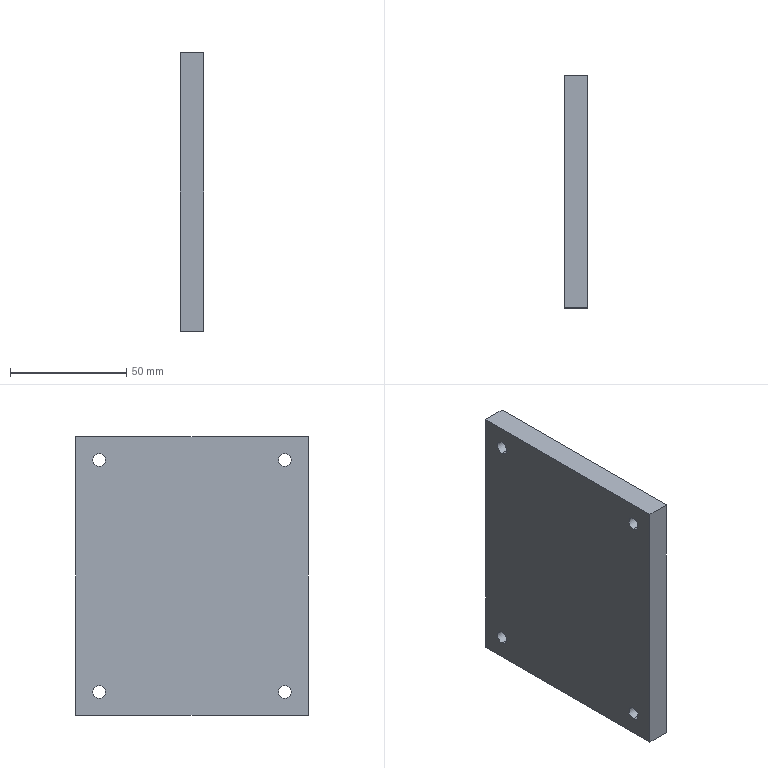Part | STEP file | A14-034 | 1 solid | 14 faces | box 10 x 100 x 120 mm | volume 119050 mm3 | cylinder 8 | plane 6 | commonest cylinder face diameters 5.5 x8
STEP:
#1=CARTESIAN_POINT('',(0.,0.,0.));
#2=DIRECTION('',(0.,0.,1.));
#3=DIRECTION('',(1.,0.,0.));
#4=AXIS2_PLACEMENT_3D('',#1,#2,#3);
#5=CARTESIAN_POINT('',(5.,40.,52.75));
#6=VERTEX_POINT('',#5);
#7=CARTESIAN_POINT('',(-5.,40.,52.75));
#8=VERTEX_POINT('',#7);
#9=CARTESIAN_POINT('',(5.,40.,52.75));
#10=DIRECTION('',(-1.,0.,0.));
#11=VECTOR('',#10,1.);
#12=LINE('',#9,#11);
#13=CARTESIAN_POINT('',(5.,40.,50.));
#14=DIRECTION('',(-1.,0.,0.));
#15=DIRECTION('',(0.,0.,1.));
#16=AXIS2_PLACEMENT_3D('',#13,#14,#15);
#17=CYLINDRICAL_SURFACE('',#16,2.75);
#18=CARTESIAN_POINT('',(6.283,0.));
#19=DIRECTION('',(0.,1.));
#20=VECTOR('',#19,1.);
#21=LINE('',#18,#20);
#22=(GEOMETRIC_REPRESENTATION_CONTEXT(2)PARAMETRIC_REPRESENTATION_CONTEXT()REPRESENTATION_CONTEXT('',''));
#23=DEFINITIONAL_REPRESENTATION('',(#21),#22);
#24=PCURVE('',#17,#23);
#25=CARTESIAN_POINT('',(5.,40.,50.));
#26=DIRECTION('',(-1.,0.,0.));
#27=DIRECTION('',(0.,0.,1.));
#28=AXIS2_PLACEMENT_3D('',#25,#26,#27);
#29=CYLINDRICAL_SURFACE('',#28,2.75);
#30=CARTESIAN_POINT('',(0.,0.));
#31=DIRECTION('',(0.,1.));
#32=VECTOR('',#31,1.);
#33=LINE('',#30,#32);
#34=(GEOMETRIC_REPRESENTATION_CONTEXT(2)PARAMETRIC_REPRESENTATION_CONTEXT()REPRESENTATION_CONTEXT('',''));
#35=DEFINITIONAL_REPRESENTATION('',(#33),#34);
#36=PCURVE('',#29,#35);
#37=SURFACE_CURVE('',#12,(#24,#36),.PCURVE_S1.);
#38=EDGE_CURVE('',#6,#8,#37,.T.);
#39=ORIENTED_EDGE('',*,*,#38,.T.);
#40=CARTESIAN_POINT('',(-5.,40.,47.25));
#41=VERTEX_POINT('',#40);
#42=CARTESIAN_POINT('',(-5.,40.,50.));
#43=DIRECTION('',(1.,0.,0.));
#44=DIRECTION('',(0.,0.,-1.));
#45=AXIS2_PLACEMENT_3D('',#42,#43,#44);
#46=CIRCLE('',#45,2.75);
#47=CARTESIAN_POINT('',(9.425,10.));
#48=DIRECTION('',(-1.,0.));
#49=VECTOR('',#48,1.);
#50=LINE('',#47,#49);
#51=(GEOMETRIC_REPRESENTATION_CONTEXT(2)PARAMETRIC_REPRESENTATION_CONTEXT()REPRESENTATION_CONTEXT('',''));
#52=DEFINITIONAL_REPRESENTATION('',(#50),#51);
#53=PCURVE('',#17,#52);
#54=CARTESIAN_POINT('',(-5.,0.,0.));
#55=DIRECTION('',(1.,0.,0.));
#56=DIRECTION('',(0.,0.,-1.));
#57=AXIS2_PLACEMENT_3D('',#54,#55,#56);
#58=PLANE('',#57);
#59=CARTESIAN_POINT('',(-50.,40.));
#60=DIRECTION('',(1.,0.));
#61=AXIS2_PLACEMENT_2D('',#59,#60);
#62=CIRCLE('',#61,2.75);
#63=(GEOMETRIC_REPRESENTATION_CONTEXT(2)PARAMETRIC_REPRESENTATION_CONTEXT()REPRESENTATION_CONTEXT('',''));
#64=DEFINITIONAL_REPRESENTATION('',(#62),#63);
#65=PCURVE('',#58,#64);
#66=SURFACE_CURVE('',#46,(#53,#65),.PCURVE_S1.);
#67=EDGE_CURVE('',#8,#41,#66,.T.);
#68=ORIENTED_EDGE('',*,*,#67,.T.);
#69=CARTESIAN_POINT('',(5.,40.,47.25));
#70=VERTEX_POINT('',#69);
#71=CARTESIAN_POINT('',(5.,40.,47.25));
#72=DIRECTION('',(-1.,0.,0.));
#73=VECTOR('',#72,1.);
#74=LINE('',#71,#73);
#75=CARTESIAN_POINT('',(3.142,0.));
#76=DIRECTION('',(0.,1.));
#77=VECTOR('',#76,1.);
#78=LINE('',#75,#77);
#79=(GEOMETRIC_REPRESENTATION_CONTEXT(2)PARAMETRIC_REPRESENTATION_CONTEXT()REPRESENTATION_CONTEXT('',''));
#80=DEFINITIONAL_REPRESENTATION('',(#78),#79);
#81=PCURVE('',#17,#80);
#82=CARTESIAN_POINT('',(3.142,0.));
#83=DIRECTION('',(0.,1.));
#84=VECTOR('',#83,1.);
#85=LINE('',#82,#84);
#86=(GEOMETRIC_REPRESENTATION_CONTEXT(2)PARAMETRIC_REPRESENTATION_CONTEXT()REPRESENTATION_CONTEXT('',''));
#87=DEFINITIONAL_REPRESENTATION('',(#85),#86);
#88=PCURVE('',#29,#87);
#89=SURFACE_CURVE('',#74,(#81,#88),.PCURVE_S1.);
#90=EDGE_CURVE('',#70,#41,#89,.T.);
#91=ORIENTED_EDGE('',*,*,#90,.F.);
#92=CARTESIAN_POINT('',(5.,40.,50.));
#93=DIRECTION('',(1.,0.,0.));
#94=DIRECTION('',(0.,0.,-1.));
#95=AXIS2_PLACEMENT_3D('',#92,#93,#94);
#96=CIRCLE('',#95,2.75);
#97=CARTESIAN_POINT('',(9.425,0.));
#98=DIRECTION('',(-1.,0.));
#99=VECTOR('',#98,1.);
#100=LINE('',#97,#99);
#101=(GEOMETRIC_REPRESENTATION_CONTEXT(2)PARAMETRIC_REPRESENTATION_CONTEXT()REPRESENTATION_CONTEXT('',''));
#102=DEFINITIONAL_REPRESENTATION('',(#100),#101);
#103=PCURVE('',#17,#102);
#104=CARTESIAN_POINT('',(5.,0.,0.));
#105=DIRECTION('',(1.,0.,0.));
#106=DIRECTION('',(0.,0.,-1.));
#107=AXIS2_PLACEMENT_3D('',#104,#105,#106);
#108=PLANE('',#107);
#109=CARTESIAN_POINT('',(-50.,40.));
#110=DIRECTION('',(1.,0.));
#111=AXIS2_PLACEMENT_2D('',#109,#110);
#112=CIRCLE('',#111,2.75);
#113=(GEOMETRIC_REPRESENTATION_CONTEXT(2)PARAMETRIC_REPRESENTATION_CONTEXT()REPRESENTATION_CONTEXT('',''));
#114=DEFINITIONAL_REPRESENTATION('',(#112),#113);
#115=PCURVE('',#108,#114);
#116=SURFACE_CURVE('',#96,(#103,#115),.PCURVE_S1.);
#117=EDGE_CURVE('',#6,#70,#116,.T.);
#118=ORIENTED_EDGE('',*,*,#117,.F.);
#119=EDGE_LOOP('',(#39,#68,#91,#118));
#120=FACE_BOUND('',#119,.F.);
#121=ADVANCED_FACE('',(#120),#17,.F.);
#122=CARTESIAN_POINT('',(5.,-40.,52.75));
#123=VERTEX_POINT('',#122);
#124=CARTESIAN_POINT('',(-5.,-40.,52.75));
#125=VERTEX_POINT('',#124);
#126=CARTESIAN_POINT('',(5.,-40.,52.75));
#127=DIRECTION('',(-1.,0.,0.));
#128=VECTOR('',#127,1.);
#129=LINE('',#126,#128);
#130=CARTESIAN_POINT('',(5.,-40.,50.));
#131=DIRECTION('',(-1.,0.,0.));
#132=DIRECTION('',(0.,0.,1.));
#133=AXIS2_PLACEMENT_3D('',#130,#131,#132);
#134=CYLINDRICAL_SURFACE('',#133,2.75);
#135=CARTESIAN_POINT('',(6.283,0.));
#136=DIRECTION('',(0.,1.));
#137=VECTOR('',#136,1.);
#138=LINE('',#135,#137);
#139=(GEOMETRIC_REPRESENTATION_CONTEXT(2)PARAMETRIC_REPRESENTATION_CONTEXT()REPRESENTATION_CONTEXT('',''));
#140=DEFINITIONAL_REPRESENTATION('',(#138),#139);
#141=PCURVE('',#134,#140);
#142=CARTESIAN_POINT('',(5.,-40.,50.));
#143=DIRECTION('',(-1.,0.,0.));
#144=DIRECTION('',(0.,0.,1.));
#145=AXIS2_PLACEMENT_3D('',#142,#143,#144);
#146=CYLINDRICAL_SURFACE('',#145,2.75);
#147=CARTESIAN_POINT('',(0.,0.));
#148=DIRECTION('',(0.,1.));
#149=VECTOR('',#148,1.);
#150=LINE('',#147,#149);
#151=(GEOMETRIC_REPRESENTATION_CONTEXT(2)PARAMETRIC_REPRESENTATION_CONTEXT()REPRESENTATION_CONTEXT('',''));
#152=DEFINITIONAL_REPRESENTATION('',(#150),#151);
#153=PCURVE('',#146,#152);
#154=SURFACE_CURVE('',#129,(#141,#153),.PCURVE_S1.);
#155=EDGE_CURVE('',#123,#125,#154,.T.);
#156=ORIENTED_EDGE('',*,*,#155,.T.);
#157=CARTESIAN_POINT('',(-5.,-40.,47.25));
#158=VERTEX_POINT('',#157);
#159=CARTESIAN_POINT('',(-5.,-40.,50.));
#160=DIRECTION('',(1.,0.,0.));
#161=DIRECTION('',(0.,0.,-1.));
#162=AXIS2_PLACEMENT_3D('',#159,#160,#161);
#163=CIRCLE('',#162,2.75);
#164=CARTESIAN_POINT('',(9.425,10.));
#165=DIRECTION('',(-1.,0.));
#166=VECTOR('',#165,1.);
#167=LINE('',#164,#166);
#168=(GEOMETRIC_REPRESENTATION_CONTEXT(2)PARAMETRIC_REPRESENTATION_CONTEXT()REPRESENTATION_CONTEXT('',''));
#169=DEFINITIONAL_REPRESENTATION('',(#167),#168);
#170=PCURVE('',#134,#169);
#171=CARTESIAN_POINT('',(-50.,-40.));
#172=DIRECTION('',(1.,0.));
#173=AXIS2_PLACEMENT_2D('',#171,#172);
#174=CIRCLE('',#173,2.75);
#175=(GEOMETRIC_REPRESENTATION_CONTEXT(2)PARAMETRIC_REPRESENTATION_CONTEXT()REPRESENTATION_CONTEXT('',''));
#176=DEFINITIONAL_REPRESENTATION('',(#174),#175);
#177=PCURVE('',#58,#176);
#178=SURFACE_CURVE('',#163,(#170,#177),.PCURVE_S1.);
#179=EDGE_CURVE('',#125,#158,#178,.T.);
#180=ORIENTED_EDGE('',*,*,#179,.T.);
#181=CARTESIAN_POINT('',(5.,-40.,47.25));
#182=VERTEX_POINT('',#181);
#183=CARTESIAN_POINT('',(5.,-40.,47.25));
#184=DIRECTION('',(-1.,0.,0.));
#185=VECTOR('',#184,1.);
#186=LINE('',#183,#185);
#187=CARTESIAN_POINT('',(3.142,0.));
#188=DIRECTION('',(0.,1.));
#189=VECTOR('',#188,1.);
#190=LINE('',#187,#189);
#191=(GEOMETRIC_REPRESENTATION_CONTEXT(2)PARAMETRIC_REPRESENTATION_CONTEXT()REPRESENTATION_CONTEXT('',''));
#192=DEFINITIONAL_REPRESENTATION('',(#190),#191);
#193=PCURVE('',#134,#192);
#194=CARTESIAN_POINT('',(3.142,0.));
#195=DIRECTION('',(0.,1.));
#196=VECTOR('',#195,1.);
#197=LINE('',#194,#196);
#198=(GEOMETRIC_REPRESENTATION_CONTEXT(2)PARAMETRIC_REPRESENTATION_CONTEXT()REPRESENTATION_CONTEXT('',''));
#199=DEFINITIONAL_REPRESENTATION('',(#197),#198);
#200=PCURVE('',#146,#199);
#201=SURFACE_CURVE('',#186,(#193,#200),.PCURVE_S1.);
#202=EDGE_CURVE('',#182,#158,#201,.T.);
#203=ORIENTED_EDGE('',*,*,#202,.F.);
#204=CARTESIAN_POINT('',(5.,-40.,50.));
#205=DIRECTION('',(1.,0.,0.));
#206=DIRECTION('',(0.,0.,-1.));
#207=AXIS2_PLACEMENT_3D('',#204,#205,#206);
#208=CIRCLE('',#207,2.75);
#209=CARTESIAN_POINT('',(9.425,0.));
#210=DIRECTION('',(-1.,0.));
#211=VECTOR('',#210,1.);
#212=LINE('',#209,#211);
#213=(GEOMETRIC_REPRESENTATION_CONTEXT(2)PARAMETRIC_REPRESENTATION_CONTEXT()REPRESENTATION_CONTEXT('',''));
#214=DEFINITIONAL_REPRESENTATION('',(#212),#213);
#215=PCURVE('',#134,#214);
#216=CARTESIAN_POINT('',(-50.,-40.));
#217=DIRECTION('',(1.,0.));
#218=AXIS2_PLACEMENT_2D('',#216,#217);
#219=CIRCLE('',#218,2.75);
#220=(GEOMETRIC_REPRESENTATION_CONTEXT(2)PARAMETRIC_REPRESENTATION_CONTEXT()REPRESENTATION_CONTEXT('',''));
#221=DEFINITIONAL_REPRESENTATION('',(#219),#220);
#222=PCURVE('',#108,#221);
#223=SURFACE_CURVE('',#208,(#215,#222),.PCURVE_S1.);
#224=EDGE_CURVE('',#123,#182,#223,.T.);
#225=ORIENTED_EDGE('',*,*,#224,.F.);
#226=EDGE_LOOP('',(#156,#180,#203,#225));
#227=FACE_BOUND('',#226,.F.);
#228=ADVANCED_FACE('',(#227),#134,.F.);
#229=CARTESIAN_POINT('',(5.,-40.,-47.25));
#230=VERTEX_POINT('',#229);
#231=CARTESIAN_POINT('',(-5.,-40.,-47.25));
#232=VERTEX_POINT('',#231);
#233=CARTESIAN_POINT('',(5.,-40.,-47.25));
#234=DIRECTION('',(-1.,0.,0.));
#235=VECTOR('',#234,1.);
#236=LINE('',#233,#235);
#237=CARTESIAN_POINT('',(5.,-40.,-50.));
#238=DIRECTION('',(-1.,0.,0.));
#239=DIRECTION('',(0.,0.,1.));
#240=AXIS2_PLACEMENT_3D('',#237,#238,#239);
#241=CYLINDRICAL_SURFACE('',#240,2.75);
#242=CARTESIAN_POINT('',(6.283,0.));
#243=DIRECTION('',(0.,1.));
#244=VECTOR('',#243,1.);
#245=LINE('',#242,#244);
#246=(GEOMETRIC_REPRESENTATION_CONTEXT(2)PARAMETRIC_REPRESENTATION_CONTEXT()REPRESENTATION_CONTEXT('',''));
#247=DEFINITIONAL_REPRESENTATION('',(#245),#246);
#248=PCURVE('',#241,#247);
#249=CARTESIAN_POINT('',(5.,-40.,-50.));
#250=DIRECTION('',(-1.,0.,0.));
#251=DIRECTION('',(0.,0.,1.));
#252=AXIS2_PLACEMENT_3D('',#249,#250,#251);
#253=CYLINDRICAL_SURFACE('',#252,2.75);
#254=CARTESIAN_POINT('',(0.,0.));
#255=DIRECTION('',(0.,1.));
#256=VECTOR('',#255,1.);
#257=LINE('',#254,#256);
#258=(GEOMETRIC_REPRESENTATION_CONTEXT(2)PARAMETRIC_REPRESENTATION_CONTEXT()REPRESENTATION_CONTEXT('',''));
#259=DEFINITIONAL_REPRESENTATION('',(#257),#258);
#260=PCURVE('',#253,#259);
#261=SURFACE_CURVE('',#236,(#248,#260),.PCURVE_S1.);
#262=EDGE_CURVE('',#230,#232,#261,.T.);
#263=ORIENTED_EDGE('',*,*,#262,.T.);
#264=CARTESIAN_POINT('',(-5.,-40.,-52.75));
#265=VERTEX_POINT('',#264);
#266=CARTESIAN_POINT('',(-5.,-40.,-50.));
#267=DIRECTION('',(1.,0.,0.));
#268=DIRECTION('',(0.,0.,-1.));
#269=AXIS2_PLACEMENT_3D('',#266,#267,#268);
#270=CIRCLE('',#269,2.75);
#271=CARTESIAN_POINT('',(9.425,10.));
#272=DIRECTION('',(-1.,0.));
#273=VECTOR('',#272,1.);
#274=LINE('',#271,#273);
#275=(GEOMETRIC_REPRESENTATION_CONTEXT(2)PARAMETRIC_REPRESENTATION_CONTEXT()REPRESENTATION_CONTEXT('',''));
#276=DEFINITIONAL_REPRESENTATION('',(#274),#275);
#277=PCURVE('',#241,#276);
#278=CARTESIAN_POINT('',(50.,-40.));
#279=DIRECTION('',(1.,0.));
#280=AXIS2_PLACEMENT_2D('',#278,#279);
#281=CIRCLE('',#280,2.75);
#282=(GEOMETRIC_REPRESENTATION_CONTEXT(2)PARAMETRIC_REPRESENTATION_CONTEXT()REPRESENTATION_CONTEXT('',''));
#283=DEFINITIONAL_REPRESENTATION('',(#281),#282);
#284=PCURVE('',#58,#283);
#285=SURFACE_CURVE('',#270,(#277,#284),.PCURVE_S1.);
#286=EDGE_CURVE('',#232,#265,#285,.T.);
#287=ORIENTED_EDGE('',*,*,#286,.T.);
#288=CARTESIAN_POINT('',(5.,-40.,-52.75));
#289=VERTEX_POINT('',#288);
#290=CARTESIAN_POINT('',(5.,-40.,-52.75));
#291=DIRECTION('',(-1.,0.,0.));
#292=VECTOR('',#291,1.);
#293=LINE('',#290,#292);
#294=CARTESIAN_POINT('',(3.142,0.));
#295=DIRECTION('',(0.,1.));
#296=VECTOR('',#295,1.);
#297=LINE('',#294,#296);
#298=(GEOMETRIC_REPRESENTATION_CONTEXT(2)PARAMETRIC_REPRESENTATION_CONTEXT()REPRESENTATION_CONTEXT('',''));
#299=DEFINITIONAL_REPRESENTATION('',(#297),#298);
#300=PCURVE('',#241,#299);
#301=CARTESIAN_POINT('',(3.142,0.));
#302=DIRECTION('',(0.,1.));
#303=VECTOR('',#302,1.);
#304=LINE('',#301,#303);
#305=(GEOMETRIC_REPRESENTATION_CONTEXT(2)PARAMETRIC_REPRESENTATION_CONTEXT()REPRESENTATION_CONTEXT('',''));
#306=DEFINITIONAL_REPRESENTATION('',(#304),#305);
#307=PCURVE('',#253,#306);
#308=SURFACE_CURVE('',#293,(#300,#307),.PCURVE_S1.);
#309=EDGE_CURVE('',#289,#265,#308,.T.);
#310=ORIENTED_EDGE('',*,*,#309,.F.);
#311=CARTESIAN_POINT('',(5.,-40.,-50.));
#312=DIRECTION('',(1.,0.,0.));
#313=DIRECTION('',(0.,0.,-1.));
#314=AXIS2_PLACEMENT_3D('',#311,#312,#313);
#315=CIRCLE('',#314,2.75);
#316=CARTESIAN_POINT('',(9.425,0.));
#317=DIRECTION('',(-1.,0.));
#318=VECTOR('',#317,1.);
#319=LINE('',#316,#318);
#320=(GEOMETRIC_REPRESENTATION_CONTEXT(2)PARAMETRIC_REPRESENTATION_CONTEXT()REPRESENTATION_CONTEXT('',''));
#321=DEFINITIONAL_REPRESENTATION('',(#319),#320);
#322=PCURVE('',#241,#321);
#323=CARTESIAN_POINT('',(50.,-40.));
#324=DIRECTION('',(1.,0.));
#325=AXIS2_PLACEMENT_2D('',#323,#324);
#326=CIRCLE('',#325,2.75);
#327=(GEOMETRIC_REPRESENTATION_CONTEXT(2)PARAMETRIC_REPRESENTATION_CONTEXT()REPRESENTATION_CONTEXT('',''));
#328=DEFINITIONAL_REPRESENTATION('',(#326),#327);
#329=PCURVE('',#108,#328);
#330=SURFACE_CURVE('',#315,(#322,#329),.PCURVE_S1.);
#331=EDGE_CURVE('',#230,#289,#330,.T.);
#332=ORIENTED_EDGE('',*,*,#331,.F.);
#333=EDGE_LOOP('',(#263,#287,#310,#332));
#334=FACE_BOUND('',#333,.F.);
#335=ADVANCED_FACE('',(#334),#241,.F.);
#336=CARTESIAN_POINT('',(5.,40.,-47.25));
#337=VERTEX_POINT('',#336);
#338=CARTESIAN_POINT('',(-5.,40.,-47.25));
#339=VERTEX_POINT('',#338);
#340=CARTESIAN_POINT('',(5.,40.,-47.25));
#341=DIRECTION('',(-1.,0.,0.));
#342=VECTOR('',#341,1.);
#343=LINE('',#340,#342);
#344=CARTESIAN_POINT('',(5.,40.,-50.));
#345=DIRECTION('',(-1.,0.,0.));
#346=DIRECTION('',(0.,0.,1.));
#347=AXIS2_PLACEMENT_3D('',#344,#345,#346);
#348=CYLINDRICAL_SURFACE('',#347,2.75);
#349=CARTESIAN_POINT('',(6.283,0.));
#350=DIRECTION('',(0.,1.));
#351=VECTOR('',#350,1.);
#352=LINE('',#349,#351);
#353=(GEOMETRIC_REPRESENTATION_CONTEXT(2)PARAMETRIC_REPRESENTATION_CONTEXT()REPRESENTATION_CONTEXT('',''));
#354=DEFINITIONAL_REPRESENTATION('',(#352),#353);
#355=PCURVE('',#348,#354);
#356=CARTESIAN_POINT('',(5.,40.,-50.));
#357=DIRECTION('',(-1.,0.,0.));
#358=DIRECTION('',(0.,0.,1.));
#359=AXIS2_PLACEMENT_3D('',#356,#357,#358);
#360=CYLINDRICAL_SURFACE('',#359,2.75);
#361=CARTESIAN_POINT('',(0.,0.));
#362=DIRECTION('',(0.,1.));
#363=VECTOR('',#362,1.);
#364=LINE('',#361,#363);
#365=(GEOMETRIC_REPRESENTATION_CONTEXT(2)PARAMETRIC_REPRESENTATION_CONTEXT()REPRESENTATION_CONTEXT('',''));
#366=DEFINITIONAL_REPRESENTATION('',(#364),#365);
#367=PCURVE('',#360,#366);
#368=SURFACE_CURVE('',#343,(#355,#367),.PCURVE_S1.);
#369=EDGE_CURVE('',#337,#339,#368,.T.);
#370=ORIENTED_EDGE('',*,*,#369,.T.);
#371=CARTESIAN_POINT('',(-5.,40.,-52.75));
#372=VERTEX_POINT('',#371);
#373=CARTESIAN_POINT('',(-5.,40.,-50.));
#374=DIRECTION('',(1.,0.,0.));
#375=DIRECTION('',(0.,0.,-1.));
#376=AXIS2_PLACEMENT_3D('',#373,#374,#375);
#377=CIRCLE('',#376,2.75);
#378=CARTESIAN_POINT('',(9.425,10.));
#379=DIRECTION('',(-1.,0.));
#380=VECTOR('',#379,1.);
#381=LINE('',#378,#380);
#382=(GEOMETRIC_REPRESENTATION_CONTEXT(2)PARAMETRIC_REPRESENTATION_CONTEXT()REPRESENTATION_CONTEXT('',''));
#383=DEFINITIONAL_REPRESENTATION('',(#381),#382);
#384=PCURVE('',#348,#383);
#385=CARTESIAN_POINT('',(50.,40.));
#386=DIRECTION('',(1.,0.));
#387=AXIS2_PLACEMENT_2D('',#385,#386);
#388=CIRCLE('',#387,2.75);
#389=(GEOMETRIC_REPRESENTATION_CONTEXT(2)PARAMETRIC_REPRESENTATION_CONTEXT()REPRESENTATION_CONTEXT('',''));
#390=DEFINITIONAL_REPRESENTATION('',(#388),#389);
#391=PCURVE('',#58,#390);
#392=SURFACE_CURVE('',#377,(#384,#391),.PCURVE_S1.);
#393=EDGE_CURVE('',#339,#372,#392,.T.);
#394=ORIENTED_EDGE('',*,*,#393,.T.);
#395=CARTESIAN_POINT('',(5.,40.,-52.75));
#396=VERTEX_POINT('',#395);
#397=CARTESIAN_POINT('',(5.,40.,-52.75));
#398=DIRECTION('',(-1.,0.,0.));
#399=VECTOR('',#398,1.);
#400=LINE('',#397,#399);
#401=CARTESIAN_POINT('',(3.142,0.));
#402=DIRECTION('',(0.,1.));
#403=VECTOR('',#402,1.);
#404=LINE('',#401,#403);
#405=(GEOMETRIC_REPRESENTATION_CONTEXT(2)PARAMETRIC_REPRESENTATION_CONTEXT()REPRESENTATION_CONTEXT('',''));
#406=DEFINITIONAL_REPRESENTATION('',(#404),#405);
#407=PCURVE('',#348,#406);
#408=CARTESIAN_POINT('',(3.142,0.));
#409=DIRECTION('',(0.,1.));
#410=VECTOR('',#409,1.);
#411=LINE('',#408,#410);
#412=(GEOMETRIC_REPRESENTATION_CONTEXT(2)PARAMETRIC_REPRESENTATION_CONTEXT()REPRESENTATION_CONTEXT('',''));
#413=DEFINITIONAL_REPRESENTATION('',(#411),#412);
#414=PCURVE('',#360,#413);
#415=SURFACE_CURVE('',#400,(#407,#414),.PCURVE_S1.);
#416=EDGE_CURVE('',#396,#372,#415,.T.);
#417=ORIENTED_EDGE('',*,*,#416,.F.);
#418=CARTESIAN_POINT('',(5.,40.,-50.));
#419=DIRECTION('',(1.,0.,0.));
#420=DIRECTION('',(0.,0.,-1.));
#421=AXIS2_PLACEMENT_3D('',#418,#419,#420);
#422=CIRCLE('',#421,2.75);
#423=CARTESIAN_POINT('',(9.425,0.));
#424=DIRECTION('',(-1.,0.));
#425=VECTOR('',#424,1.);
#426=LINE('',#423,#425);
#427=(GEOMETRIC_REPRESENTATION_CONTEXT(2)PARAMETRIC_REPRESENTATION_CONTEXT()REPRESENTATION_CONTEXT('',''));
#428=DEFINITIONAL_REPRESENTATION('',(#426),#427);
#429=PCURVE('',#348,#428);
#430=CARTESIAN_POINT('',(50.,40.));
#431=DIRECTION('',(1.,0.));
#432=AXIS2_PLACEMENT_2D('',#430,#431);
#433=CIRCLE('',#432,2.75);
#434=(GEOMETRIC_REPRESENTATION_CONTEXT(2)PARAMETRIC_REPRESENTATION_CONTEXT()REPRESENTATION_CONTEXT('',''));
#435=DEFINITIONAL_REPRESENTATION('',(#433),#434);
#436=PCURVE('',#108,#435);
#437=SURFACE_CURVE('',#422,(#429,#436),.PCURVE_S1.);
#438=EDGE_CURVE('',#337,#396,#437,.T.);
#439=ORIENTED_EDGE('',*,*,#438,.F.);
#440=EDGE_LOOP('',(#370,#394,#417,#439));
#441=FACE_BOUND('',#440,.F.);
#442=ADVANCED_FACE('',(#441),#348,.F.);
#443=ORIENTED_EDGE('',*,*,#224,.F.);
#444=CARTESIAN_POINT('',(5.,-40.,50.));
#445=DIRECTION('',(1.,0.,0.));
#446=DIRECTION('',(0.,0.,-1.));
#447=AXIS2_PLACEMENT_3D('',#444,#445,#446);
#448=CIRCLE('',#447,2.75);
#449=CARTESIAN_POINT('',(-50.,-40.));
#450=DIRECTION('',(1.,0.));
#451=AXIS2_PLACEMENT_2D('',#449,#450);
#452=CIRCLE('',#451,2.75);
#453=(GEOMETRIC_REPRESENTATION_CONTEXT(2)PARAMETRIC_REPRESENTATION_CONTEXT()REPRESENTATION_CONTEXT('',''));
#454=DEFINITIONAL_REPRESENTATION('',(#452),#453);
#455=PCURVE('',#108,#454);
#456=CARTESIAN_POINT('',(3.142,0.));
#457=DIRECTION('',(-1.,0.));
#458=VECTOR('',#457,1.);
#459=LINE('',#456,#458);
#460=(GEOMETRIC_REPRESENTATION_CONTEXT(2)PARAMETRIC_REPRESENTATION_CONTEXT()REPRESENTATION_CONTEXT('',''));
#461=DEFINITIONAL_REPRESENTATION('',(#459),#460);
#462=PCURVE('',#146,#461);
#463=SURFACE_CURVE('',#448,(#455,#462),.PCURVE_S1.);
#464=EDGE_CURVE('',#182,#123,#463,.T.);
#465=ORIENTED_EDGE('',*,*,#464,.F.);
#466=EDGE_LOOP('',(#443,#465));
#467=FACE_BOUND('',#466,.T.);
#468=ORIENTED_EDGE('',*,*,#438,.F.);
#469=CARTESIAN_POINT('',(5.,40.,-50.));
#470=DIRECTION('',(1.,0.,0.));
#471=DIRECTION('',(0.,0.,-1.));
#472=AXIS2_PLACEMENT_3D('',#469,#470,#471);
#473=CIRCLE('',#472,2.75);
#474=CARTESIAN_POINT('',(50.,40.));
#475=DIRECTION('',(1.,0.));
#476=AXIS2_PLACEMENT_2D('',#474,#475);
#477=CIRCLE('',#476,2.75);
#478=(GEOMETRIC_REPRESENTATION_CONTEXT(2)PARAMETRIC_REPRESENTATION_CONTEXT()REPRESENTATION_CONTEXT('',''));
#479=DEFINITIONAL_REPRESENTATION('',(#477),#478);
#480=PCURVE('',#108,#479);
#481=CARTESIAN_POINT('',(3.142,0.));
#482=DIRECTION('',(-1.,0.));
#483=VECTOR('',#482,1.);
#484=LINE('',#481,#483);
#485=(GEOMETRIC_REPRESENTATION_CONTEXT(2)PARAMETRIC_REPRESENTATION_CONTEXT()REPRESENTATION_CONTEXT('',''));
#486=DEFINITIONAL_REPRESENTATION('',(#484),#485);
#487=PCURVE('',#360,#486);
#488=SURFACE_CURVE('',#473,(#480,#487),.PCURVE_S1.);
#489=EDGE_CURVE('',#396,#337,#488,.T.);
#490=ORIENTED_EDGE('',*,*,#489,.F.);
#491=EDGE_LOOP('',(#468,#490));
#492=FACE_BOUND('',#491,.T.);
#493=CARTESIAN_POINT('',(5.,-50.,-60.));
#494=VERTEX_POINT('',#493);
#495=CARTESIAN_POINT('',(5.,50.,-60.));
#496=VERTEX_POINT('',#495);
#497=CARTESIAN_POINT('',(5.,50.,-60.));
#498=DIRECTION('',(0.,1.,0.));
#499=VECTOR('',#498,1.);
#500=LINE('',#497,#499);
#501=CARTESIAN_POINT('',(60.,50.));
#502=DIRECTION('',(0.,1.));
#503=VECTOR('',#502,1.);
#504=LINE('',#501,#503);
#505=(GEOMETRIC_REPRESENTATION_CONTEXT(2)PARAMETRIC_REPRESENTATION_CONTEXT()REPRESENTATION_CONTEXT('',''));
#506=DEFINITIONAL_REPRESENTATION('',(#504),#505);
#507=PCURVE('',#108,#506);
#508=CARTESIAN_POINT('',(5.,50.,-60.));
#509=DIRECTION('',(0.,0.,1.));
#510=DIRECTION('',(1.,0.,0.));
#511=AXIS2_PLACEMENT_3D('',#508,#509,#510);
#512=PLANE('',#511);
#513=CARTESIAN_POINT('',(0.,0.));
#514=DIRECTION('',(0.,1.));
#515=VECTOR('',#514,1.);
#516=LINE('',#513,#515);
#517=(GEOMETRIC_REPRESENTATION_CONTEXT(2)PARAMETRIC_REPRESENTATION_CONTEXT()REPRESENTATION_CONTEXT('',''));
#518=DEFINITIONAL_REPRESENTATION('',(#516),#517);
#519=PCURVE('',#512,#518);
#520=SURFACE_CURVE('',#500,(#507,#519),.PCURVE_S1.);
#521=EDGE_CURVE('',#494,#496,#520,.T.);
#522=ORIENTED_EDGE('',*,*,#521,.T.);
#523=CARTESIAN_POINT('',(5.,50.,60.));
#524=VERTEX_POINT('',#523);
#525=CARTESIAN_POINT('',(5.,50.,60.));
#526=DIRECTION('',(0.,0.,1.));
#527=VECTOR('',#526,1.);
#528=LINE('',#525,#527);
#529=CARTESIAN_POINT('',(-60.,50.));
#530=DIRECTION('',(-1.,0.));
#531=VECTOR('',#530,1.);
#532=LINE('',#529,#531);
#533=(GEOMETRIC_REPRESENTATION_CONTEXT(2)PARAMETRIC_REPRESENTATION_CONTEXT()REPRESENTATION_CONTEXT('',''));
#534=DEFINITIONAL_REPRESENTATION('',(#532),#533);
#535=PCURVE('',#108,#534);
#536=CARTESIAN_POINT('',(5.,50.,60.));
#537=DIRECTION('',(0.,-1.,0.));
#538=DIRECTION('',(0.,0.,-1.));
#539=AXIS2_PLACEMENT_3D('',#536,#537,#538);
#540=PLANE('',#539);
#541=CARTESIAN_POINT('',(0.,0.));
#542=DIRECTION('',(-1.,0.));
#543=VECTOR('',#542,1.);
#544=LINE('',#541,#543);
#545=(GEOMETRIC_REPRESENTATION_CONTEXT(2)PARAMETRIC_REPRESENTATION_CONTEXT()REPRESENTATION_CONTEXT('',''));
#546=DEFINITIONAL_REPRESENTATION('',(#544),#545);
#547=PCURVE('',#540,#546);
#548=SURFACE_CURVE('',#528,(#535,#547),.PCURVE_S1.);
#549=EDGE_CURVE('',#496,#524,#548,.T.);
#550=ORIENTED_EDGE('',*,*,#549,.T.);
#551=CARTESIAN_POINT('',(5.,-50.,60.));
#552=VERTEX_POINT('',#551);
#553=CARTESIAN_POINT('',(5.,50.,60.));
#554=DIRECTION('',(0.,-1.,0.));
#555=VECTOR('',#554,1.);
#556=LINE('',#553,#555);
#557=CARTESIAN_POINT('',(-60.,50.));
#558=DIRECTION('',(0.,-1.));
#559=VECTOR('',#558,1.);
#560=LINE('',#557,#559);
#561=(GEOMETRIC_REPRESENTATION_CONTEXT(2)PARAMETRIC_REPRESENTATION_CONTEXT()REPRESENTATION_CONTEXT('',''));
#562=DEFINITIONAL_REPRESENTATION('',(#560),#561);
#563=PCURVE('',#108,#562);
#564=CARTESIAN_POINT('',(5.,50.,60.));
#565=DIRECTION('',(0.,0.,-1.));
#566=DIRECTION('',(-1.,0.,0.));
#567=AXIS2_PLACEMENT_3D('',#564,#565,#566);
#568=PLANE('',#567);
#569=CARTESIAN_POINT('',(0.,0.));
#570=DIRECTION('',(0.,-1.));
#571=VECTOR('',#570,1.);
#572=LINE('',#569,#571);
#573=(GEOMETRIC_REPRESENTATION_CONTEXT(2)PARAMETRIC_REPRESENTATION_CONTEXT()REPRESENTATION_CONTEXT('',''));
#574=DEFINITIONAL_REPRESENTATION('',(#572),#573);
#575=PCURVE('',#568,#574);
#576=SURFACE_CURVE('',#556,(#563,#575),.PCURVE_S1.);
#577=EDGE_CURVE('',#524,#552,#576,.T.);
#578=ORIENTED_EDGE('',*,*,#577,.T.);
#579=CARTESIAN_POINT('',(5.,-50.,60.));
#580=DIRECTION('',(0.,0.,-1.));
#581=VECTOR('',#580,1.);
#582=LINE('',#579,#581);
#583=CARTESIAN_POINT('',(-60.,-50.));
#584=DIRECTION('',(1.,0.));
#585=VECTOR('',#584,1.);
#586=LINE('',#583,#585);
#587=(GEOMETRIC_REPRESENTATION_CONTEXT(2)PARAMETRIC_REPRESENTATION_CONTEXT()REPRESENTATION_CONTEXT('',''));
#588=DEFINITIONAL_REPRESENTATION('',(#586),#587);
#589=PCURVE('',#108,#588);
#590=CARTESIAN_POINT('',(5.,-50.,60.));
#591=DIRECTION('',(0.,1.,0.));
#592=DIRECTION('',(0.,0.,1.));
#593=AXIS2_PLACEMENT_3D('',#590,#591,#592);
#594=PLANE('',#593);
#595=CARTESIAN_POINT('',(0.,0.));
#596=DIRECTION('',(-1.,0.));
#597=VECTOR('',#596,1.);
#598=LINE('',#595,#597);
#599=(GEOMETRIC_REPRESENTATION_CONTEXT(2)PARAMETRIC_REPRESENTATION_CONTEXT()REPRESENTATION_CONTEXT('',''));
#600=DEFINITIONAL_REPRESENTATION('',(#598),#599);
#601=PCURVE('',#594,#600);
#602=SURFACE_CURVE('',#582,(#589,#601),.PCURVE_S1.);
#603=EDGE_CURVE('',#552,#494,#602,.T.);
#604=ORIENTED_EDGE('',*,*,#603,.T.);
#605=EDGE_LOOP('',(#522,#550,#578,#604));
#606=FACE_BOUND('',#605,.T.);
#607=ORIENTED_EDGE('',*,*,#331,.F.);
#608=CARTESIAN_POINT('',(5.,-40.,-50.));
#609=DIRECTION('',(1.,0.,0.));
#610=DIRECTION('',(0.,0.,-1.));
#611=AXIS2_PLACEMENT_3D('',#608,#609,#610);
#612=CIRCLE('',#611,2.75);
#613=CARTESIAN_POINT('',(50.,-40.));
#614=DIRECTION('',(1.,0.));
#615=AXIS2_PLACEMENT_2D('',#613,#614);
#616=CIRCLE('',#615,2.75);
#617=(GEOMETRIC_REPRESENTATION_CONTEXT(2)PARAMETRIC_REPRESENTATION_CONTEXT()REPRESENTATION_CONTEXT('',''));
#618=DEFINITIONAL_REPRESENTATION('',(#616),#617);
#619=PCURVE('',#108,#618);
#620=CARTESIAN_POINT('',(3.142,0.));
#621=DIRECTION('',(-1.,0.));
#622=VECTOR('',#621,1.);
#623=LINE('',#620,#622);
#624=(GEOMETRIC_REPRESENTATION_CONTEXT(2)PARAMETRIC_REPRESENTATION_CONTEXT()REPRESENTATION_CONTEXT('',''));
#625=DEFINITIONAL_REPRESENTATION('',(#623),#624);
#626=PCURVE('',#253,#625);
#627=SURFACE_CURVE('',#612,(#619,#626),.PCURVE_S1.);
#628=EDGE_CURVE('',#289,#230,#627,.T.);
#629=ORIENTED_EDGE('',*,*,#628,.F.);
#630=EDGE_LOOP('',(#607,#629));
#631=FACE_BOUND('',#630,.T.);
#632=ORIENTED_EDGE('',*,*,#117,.F.);
#633=CARTESIAN_POINT('',(5.,40.,50.));
#634=DIRECTION('',(1.,0.,0.));
#635=DIRECTION('',(0.,0.,-1.));
#636=AXIS2_PLACEMENT_3D('',#633,#634,#635);
#637=CIRCLE('',#636,2.75);
#638=CARTESIAN_POINT('',(-50.,40.));
#639=DIRECTION('',(1.,0.));
#640=AXIS2_PLACEMENT_2D('',#638,#639);
#641=CIRCLE('',#640,2.75);
#642=(GEOMETRIC_REPRESENTATION_CONTEXT(2)PARAMETRIC_REPRESENTATION_CONTEXT()REPRESENTATION_CONTEXT('',''));
#643=DEFINITIONAL_REPRESENTATION('',(#641),#642);
#644=PCURVE('',#108,#643);
#645=CARTESIAN_POINT('',(3.142,0.));
#646=DIRECTION('',(-1.,0.));
#647=VECTOR('',#646,1.);
#648=LINE('',#645,#647);
#649=(GEOMETRIC_REPRESENTATION_CONTEXT(2)PARAMETRIC_REPRESENTATION_CONTEXT()REPRESENTATION_CONTEXT('',''));
#650=DEFINITIONAL_REPRESENTATION('',(#648),#649);
#651=PCURVE('',#29,#650);
#652=SURFACE_CURVE('',#637,(#644,#651),.PCURVE_S1.);
#653=EDGE_CURVE('',#70,#6,#652,.T.);
#654=ORIENTED_EDGE('',*,*,#653,.F.);
#655=EDGE_LOOP('',(#632,#654));
#656=FACE_BOUND('',#655,.T.);
#657=ADVANCED_FACE('',(#467,#492,#606,#631,#656),#108,.T.);
#658=CARTESIAN_POINT('',(-5.,-50.,-60.));
#659=VERTEX_POINT('',#658);
#660=CARTESIAN_POINT('',(-5.,50.,-60.));
#661=VERTEX_POINT('',#660);
#662=CARTESIAN_POINT('',(-5.,50.,-60.));
#663=DIRECTION('',(0.,1.,0.));
#664=VECTOR('',#663,1.);
#665=LINE('',#662,#664);
#666=CARTESIAN_POINT('',(60.,50.));
#667=DIRECTION('',(0.,1.));
#668=VECTOR('',#667,1.);
#669=LINE('',#666,#668);
#670=(GEOMETRIC_REPRESENTATION_CONTEXT(2)PARAMETRIC_REPRESENTATION_CONTEXT()REPRESENTATION_CONTEXT('',''));
#671=DEFINITIONAL_REPRESENTATION('',(#669),#670);
#672=PCURVE('',#58,#671);
#673=CARTESIAN_POINT('',(-10.,0.));
#674=DIRECTION('',(0.,1.));
#675=VECTOR('',#674,1.);
#676=LINE('',#673,#675);
#677=(GEOMETRIC_REPRESENTATION_CONTEXT(2)PARAMETRIC_REPRESENTATION_CONTEXT()REPRESENTATION_CONTEXT('',''));
#678=DEFINITIONAL_REPRESENTATION('',(#676),#677);
#679=PCURVE('',#512,#678);
#680=SURFACE_CURVE('',#665,(#672,#679),.PCURVE_S1.);
#681=EDGE_CURVE('',#659,#661,#680,.T.);
#682=ORIENTED_EDGE('',*,*,#681,.F.);
#683=CARTESIAN_POINT('',(-5.,-50.,60.));
#684=VERTEX_POINT('',#683);
#685=CARTESIAN_POINT('',(-5.,-50.,60.));
#686=DIRECTION('',(0.,0.,-1.));
#687=VECTOR('',#686,1.);
#688=LINE('',#685,#687);
#689=CARTESIAN_POINT('',(-60.,-50.));
#690=DIRECTION('',(1.,0.));
#691=VECTOR('',#690,1.);
#692=LINE('',#689,#691);
#693=(GEOMETRIC_REPRESENTATION_CONTEXT(2)PARAMETRIC_REPRESENTATION_CONTEXT()REPRESENTATION_CONTEXT('',''));
#694=DEFINITIONAL_REPRESENTATION('',(#692),#693);
#695=PCURVE('',#58,#694);
#696=CARTESIAN_POINT('',(0.,-10.));
#697=DIRECTION('',(-1.,0.));
#698=VECTOR('',#697,1.);
#699=LINE('',#696,#698);
#700=(GEOMETRIC_REPRESENTATION_CONTEXT(2)PARAMETRIC_REPRESENTATION_CONTEXT()REPRESENTATION_CONTEXT('',''));
#701=DEFINITIONAL_REPRESENTATION('',(#699),#700);
#702=PCURVE('',#594,#701);
#703=SURFACE_CURVE('',#688,(#695,#702),.PCURVE_S1.);
#704=EDGE_CURVE('',#684,#659,#703,.T.);
#705=ORIENTED_EDGE('',*,*,#704,.F.);
#706=CARTESIAN_POINT('',(-5.,50.,60.));
#707=VERTEX_POINT('',#706);
#708=CARTESIAN_POINT('',(-5.,50.,60.));
#709=DIRECTION('',(0.,-1.,0.));
#710=VECTOR('',#709,1.);
#711=LINE('',#708,#710);
#712=CARTESIAN_POINT('',(-60.,50.));
#713=DIRECTION('',(0.,-1.));
#714=VECTOR('',#713,1.);
#715=LINE('',#712,#714);
#716=(GEOMETRIC_REPRESENTATION_CONTEXT(2)PARAMETRIC_REPRESENTATION_CONTEXT()REPRESENTATION_CONTEXT('',''));
#717=DEFINITIONAL_REPRESENTATION('',(#715),#716);
#718=PCURVE('',#58,#717);
#719=CARTESIAN_POINT('',(10.,0.));
#720=DIRECTION('',(0.,-1.));
#721=VECTOR('',#720,1.);
#722=LINE('',#719,#721);
#723=(GEOMETRIC_REPRESENTATION_CONTEXT(2)PARAMETRIC_REPRESENTATION_CONTEXT()REPRESENTATION_CONTEXT('',''));
#724=DEFINITIONAL_REPRESENTATION('',(#722),#723);
#725=PCURVE('',#568,#724);
#726=SURFACE_CURVE('',#711,(#718,#725),.PCURVE_S1.);
#727=EDGE_CURVE('',#707,#684,#726,.T.);
#728=ORIENTED_EDGE('',*,*,#727,.F.);
#729=CARTESIAN_POINT('',(-5.,50.,60.));
#730=DIRECTION('',(0.,0.,1.));
#731=VECTOR('',#730,1.);
#732=LINE('',#729,#731);
#733=CARTESIAN_POINT('',(-60.,50.));
#734=DIRECTION('',(-1.,0.));
#735=VECTOR('',#734,1.);
#736=LINE('',#733,#735);
#737=(GEOMETRIC_REPRESENTATION_CONTEXT(2)PARAMETRIC_REPRESENTATION_CONTEXT()REPRESENTATION_CONTEXT('',''));
#738=DEFINITIONAL_REPRESENTATION('',(#736),#737);
#739=PCURVE('',#58,#738);
#740=CARTESIAN_POINT('',(0.,-10.));
#741=DIRECTION('',(-1.,0.));
#742=VECTOR('',#741,1.);
#743=LINE('',#740,#742);
#744=(GEOMETRIC_REPRESENTATION_CONTEXT(2)PARAMETRIC_REPRESENTATION_CONTEXT()REPRESENTATION_CONTEXT('',''));
#745=DEFINITIONAL_REPRESENTATION('',(#743),#744);
#746=PCURVE('',#540,#745);
#747=SURFACE_CURVE('',#732,(#739,#746),.PCURVE_S1.);
#748=EDGE_CURVE('',#661,#707,#747,.T.);
#749=ORIENTED_EDGE('',*,*,#748,.F.);
#750=EDGE_LOOP('',(#682,#705,#728,#749));
#751=FACE_BOUND('',#750,.T.);
#752=ORIENTED_EDGE('',*,*,#393,.T.);
#753=CARTESIAN_POINT('',(-5.,40.,-50.));
#754=DIRECTION('',(1.,0.,0.));
#755=DIRECTION('',(0.,0.,-1.));
#756=AXIS2_PLACEMENT_3D('',#753,#754,#755);
#757=CIRCLE('',#756,2.75);
#758=CARTESIAN_POINT('',(50.,40.));
#759=DIRECTION('',(1.,0.));
#760=AXIS2_PLACEMENT_2D('',#758,#759);
#761=CIRCLE('',#760,2.75);
#762=(GEOMETRIC_REPRESENTATION_CONTEXT(2)PARAMETRIC_REPRESENTATION_CONTEXT()REPRESENTATION_CONTEXT('',''));
#763=DEFINITIONAL_REPRESENTATION('',(#761),#762);
#764=PCURVE('',#58,#763);
#765=CARTESIAN_POINT('',(3.142,10.));
#766=DIRECTION('',(-1.,0.));
#767=VECTOR('',#766,1.);
#768=LINE('',#765,#767);
#769=(GEOMETRIC_REPRESENTATION_CONTEXT(2)PARAMETRIC_REPRESENTATION_CONTEXT()REPRESENTATION_CONTEXT('',''));
#770=DEFINITIONAL_REPRESENTATION('',(#768),#769);
#771=PCURVE('',#360,#770);
#772=SURFACE_CURVE('',#757,(#764,#771),.PCURVE_S1.);
#773=EDGE_CURVE('',#372,#339,#772,.T.);
#774=ORIENTED_EDGE('',*,*,#773,.T.);
#775=EDGE_LOOP('',(#752,#774));
#776=FACE_BOUND('',#775,.T.);
#777=ORIENTED_EDGE('',*,*,#286,.T.);
#778=CARTESIAN_POINT('',(-5.,-40.,-50.));
#779=DIRECTION('',(1.,0.,0.));
#780=DIRECTION('',(0.,0.,-1.));
#781=AXIS2_PLACEMENT_3D('',#778,#779,#780);
#782=CIRCLE('',#781,2.75);
#783=CARTESIAN_POINT('',(50.,-40.));
#784=DIRECTION('',(1.,0.));
#785=AXIS2_PLACEMENT_2D('',#783,#784);
#786=CIRCLE('',#785,2.75);
#787=(GEOMETRIC_REPRESENTATION_CONTEXT(2)PARAMETRIC_REPRESENTATION_CONTEXT()REPRESENTATION_CONTEXT('',''));
#788=DEFINITIONAL_REPRESENTATION('',(#786),#787);
#789=PCURVE('',#58,#788);
#790=CARTESIAN_POINT('',(3.142,10.));
#791=DIRECTION('',(-1.,0.));
#792=VECTOR('',#791,1.);
#793=LINE('',#790,#792);
#794=(GEOMETRIC_REPRESENTATION_CONTEXT(2)PARAMETRIC_REPRESENTATION_CONTEXT()REPRESENTATION_CONTEXT('',''));
#795=DEFINITIONAL_REPRESENTATION('',(#793),#794);
#796=PCURVE('',#253,#795);
#797=SURFACE_CURVE('',#782,(#789,#796),.PCURVE_S1.);
#798=EDGE_CURVE('',#265,#232,#797,.T.);
#799=ORIENTED_EDGE('',*,*,#798,.T.);
#800=EDGE_LOOP('',(#777,#799));
#801=FACE_BOUND('',#800,.T.);
#802=ORIENTED_EDGE('',*,*,#179,.T.);
#803=CARTESIAN_POINT('',(-5.,-40.,50.));
#804=DIRECTION('',(1.,0.,0.));
#805=DIRECTION('',(0.,0.,-1.));
#806=AXIS2_PLACEMENT_3D('',#803,#804,#805);
#807=CIRCLE('',#806,2.75);
#808=CARTESIAN_POINT('',(-50.,-40.));
#809=DIRECTION('',(1.,0.));
#810=AXIS2_PLACEMENT_2D('',#808,#809);
#811=CIRCLE('',#810,2.75);
#812=(GEOMETRIC_REPRESENTATION_CONTEXT(2)PARAMETRIC_REPRESENTATION_CONTEXT()REPRESENTATION_CONTEXT('',''));
#813=DEFINITIONAL_REPRESENTATION('',(#811),#812);
#814=PCURVE('',#58,#813);
#815=CARTESIAN_POINT('',(3.142,10.));
#816=DIRECTION('',(-1.,0.));
#817=VECTOR('',#816,1.);
#818=LINE('',#815,#817);
#819=(GEOMETRIC_REPRESENTATION_CONTEXT(2)PARAMETRIC_REPRESENTATION_CONTEXT()REPRESENTATION_CONTEXT('',''));
#820=DEFINITIONAL_REPRESENTATION('',(#818),#819);
#821=PCURVE('',#146,#820);
#822=SURFACE_CURVE('',#807,(#814,#821),.PCURVE_S1.);
#823=EDGE_CURVE('',#158,#125,#822,.T.);
#824=ORIENTED_EDGE('',*,*,#823,.T.);
#825=EDGE_LOOP('',(#802,#824));
#826=FACE_BOUND('',#825,.T.);
#827=ORIENTED_EDGE('',*,*,#67,.T.);
#828=CARTESIAN_POINT('',(-5.,40.,50.));
#829=DIRECTION('',(1.,0.,0.));
#830=DIRECTION('',(0.,0.,-1.));
#831=AXIS2_PLACEMENT_3D('',#828,#829,#830);
#832=CIRCLE('',#831,2.75);
#833=CARTESIAN_POINT('',(-50.,40.));
#834=DIRECTION('',(1.,0.));
#835=AXIS2_PLACEMENT_2D('',#833,#834);
#836=CIRCLE('',#835,2.75);
#837=(GEOMETRIC_REPRESENTATION_CONTEXT(2)PARAMETRIC_REPRESENTATION_CONTEXT()REPRESENTATION_CONTEXT('',''));
#838=DEFINITIONAL_REPRESENTATION('',(#836),#837);
#839=PCURVE('',#58,#838);
#840=CARTESIAN_POINT('',(3.142,10.));
#841=DIRECTION('',(-1.,0.));
#842=VECTOR('',#841,1.);
#843=LINE('',#840,#842);
#844=(GEOMETRIC_REPRESENTATION_CONTEXT(2)PARAMETRIC_REPRESENTATION_CONTEXT()REPRESENTATION_CONTEXT('',''));
#845=DEFINITIONAL_REPRESENTATION('',(#843),#844);
#846=PCURVE('',#29,#845);
#847=SURFACE_CURVE('',#832,(#839,#846),.PCURVE_S1.);
#848=EDGE_CURVE('',#41,#8,#847,.T.);
#849=ORIENTED_EDGE('',*,*,#848,.T.);
#850=EDGE_LOOP('',(#827,#849));
#851=FACE_BOUND('',#850,.T.);
#852=ADVANCED_FACE('',(#751,#776,#801,#826,#851),#58,.F.);
#853=ORIENTED_EDGE('',*,*,#681,.T.);
#854=CARTESIAN_POINT('',(5.,50.,-60.));
#855=DIRECTION('',(-1.,0.,0.));
#856=VECTOR('',#855,1.);
#857=LINE('',#854,#856);
#858=CARTESIAN_POINT('',(0.,0.));
#859=DIRECTION('',(-1.,0.));
#860=VECTOR('',#859,1.);
#861=LINE('',#858,#860);
#862=(GEOMETRIC_REPRESENTATION_CONTEXT(2)PARAMETRIC_REPRESENTATION_CONTEXT()REPRESENTATION_CONTEXT('',''));
#863=DEFINITIONAL_REPRESENTATION('',(#861),#862);
#864=PCURVE('',#512,#863);
#865=CARTESIAN_POINT('',(120.,0.));
#866=DIRECTION('',(0.,-1.));
#867=VECTOR('',#866,1.);
#868=LINE('',#865,#867);
#869=(GEOMETRIC_REPRESENTATION_CONTEXT(2)PARAMETRIC_REPRESENTATION_CONTEXT()REPRESENTATION_CONTEXT('',''));
#870=DEFINITIONAL_REPRESENTATION('',(#868),#869);
#871=PCURVE('',#540,#870);
#872=SURFACE_CURVE('',#857,(#864,#871),.PCURVE_S1.);
#873=EDGE_CURVE('',#496,#661,#872,.T.);
#874=ORIENTED_EDGE('',*,*,#873,.F.);
#875=ORIENTED_EDGE('',*,*,#521,.F.);
#876=CARTESIAN_POINT('',(5.,-50.,-60.));
#877=DIRECTION('',(-1.,0.,0.));
#878=VECTOR('',#877,1.);
#879=LINE('',#876,#878);
#880=CARTESIAN_POINT('',(0.,-100.));
#881=DIRECTION('',(-1.,0.));
#882=VECTOR('',#881,1.);
#883=LINE('',#880,#882);
#884=(GEOMETRIC_REPRESENTATION_CONTEXT(2)PARAMETRIC_REPRESENTATION_CONTEXT()REPRESENTATION_CONTEXT('',''));
#885=DEFINITIONAL_REPRESENTATION('',(#883),#884);
#886=PCURVE('',#512,#885);
#887=CARTESIAN_POINT('',(-120.,0.));
#888=DIRECTION('',(0.,-1.));
#889=VECTOR('',#888,1.);
#890=LINE('',#887,#889);
#891=(GEOMETRIC_REPRESENTATION_CONTEXT(2)PARAMETRIC_REPRESENTATION_CONTEXT()REPRESENTATION_CONTEXT('',''));
#892=DEFINITIONAL_REPRESENTATION('',(#890),#891);
#893=PCURVE('',#594,#892);
#894=SURFACE_CURVE('',#879,(#886,#893),.PCURVE_S1.);
#895=EDGE_CURVE('',#494,#659,#894,.T.);
#896=ORIENTED_EDGE('',*,*,#895,.T.);
#897=EDGE_LOOP('',(#853,#874,#875,#896));
#898=FACE_BOUND('',#897,.T.);
#899=ADVANCED_FACE('',(#898),#512,.F.);
#900=ORIENTED_EDGE('',*,*,#748,.T.);
#901=CARTESIAN_POINT('',(5.,50.,60.));
#902=DIRECTION('',(-1.,0.,0.));
#903=VECTOR('',#902,1.);
#904=LINE('',#901,#903);
#905=CARTESIAN_POINT('',(0.,0.));
#906=DIRECTION('',(0.,-1.));
#907=VECTOR('',#906,1.);
#908=LINE('',#905,#907);
#909=(GEOMETRIC_REPRESENTATION_CONTEXT(2)PARAMETRIC_REPRESENTATION_CONTEXT()REPRESENTATION_CONTEXT('',''));
#910=DEFINITIONAL_REPRESENTATION('',(#908),#909);
#911=PCURVE('',#540,#910);
#912=CARTESIAN_POINT('',(0.,0.));
#913=DIRECTION('',(1.,0.));
#914=VECTOR('',#913,1.);
#915=LINE('',#912,#914);
#916=(GEOMETRIC_REPRESENTATION_CONTEXT(2)PARAMETRIC_REPRESENTATION_CONTEXT()REPRESENTATION_CONTEXT('',''));
#917=DEFINITIONAL_REPRESENTATION('',(#915),#916);
#918=PCURVE('',#568,#917);
#919=SURFACE_CURVE('',#904,(#911,#918),.PCURVE_S1.);
#920=EDGE_CURVE('',#524,#707,#919,.T.);
#921=ORIENTED_EDGE('',*,*,#920,.F.);
#922=ORIENTED_EDGE('',*,*,#549,.F.);
#923=ORIENTED_EDGE('',*,*,#873,.T.);
#924=EDGE_LOOP('',(#900,#921,#922,#923));
#925=FACE_BOUND('',#924,.T.);
#926=ADVANCED_FACE('',(#925),#540,.F.);
#927=ORIENTED_EDGE('',*,*,#727,.T.);
#928=CARTESIAN_POINT('',(5.,-50.,60.));
#929=DIRECTION('',(-1.,0.,0.));
#930=VECTOR('',#929,1.);
#931=LINE('',#928,#930);
#932=CARTESIAN_POINT('',(0.,-100.));
#933=DIRECTION('',(1.,0.));
#934=VECTOR('',#933,1.);
#935=LINE('',#932,#934);
#936=(GEOMETRIC_REPRESENTATION_CONTEXT(2)PARAMETRIC_REPRESENTATION_CONTEXT()REPRESENTATION_CONTEXT('',''));
#937=DEFINITIONAL_REPRESENTATION('',(#935),#936);
#938=PCURVE('',#568,#937);
#939=CARTESIAN_POINT('',(0.,0.));
#940=DIRECTION('',(0.,-1.));
#941=VECTOR('',#940,1.);
#942=LINE('',#939,#941);
#943=(GEOMETRIC_REPRESENTATION_CONTEXT(2)PARAMETRIC_REPRESENTATION_CONTEXT()REPRESENTATION_CONTEXT('',''));
#944=DEFINITIONAL_REPRESENTATION('',(#942),#943);
#945=PCURVE('',#594,#944);
#946=SURFACE_CURVE('',#931,(#938,#945),.PCURVE_S1.);
#947=EDGE_CURVE('',#552,#684,#946,.T.);
#948=ORIENTED_EDGE('',*,*,#947,.F.);
#949=ORIENTED_EDGE('',*,*,#577,.F.);
#950=ORIENTED_EDGE('',*,*,#920,.T.);
#951=EDGE_LOOP('',(#927,#948,#949,#950));
#952=FACE_BOUND('',#951,.T.);
#953=ADVANCED_FACE('',(#952),#568,.F.);
#954=ORIENTED_EDGE('',*,*,#704,.T.);
#955=ORIENTED_EDGE('',*,*,#895,.F.);
#956=ORIENTED_EDGE('',*,*,#603,.F.);
#957=ORIENTED_EDGE('',*,*,#947,.T.);
#958=EDGE_LOOP('',(#954,#955,#956,#957));
#959=FACE_BOUND('',#958,.T.);
#960=ADVANCED_FACE('',(#959),#594,.F.);
#961=ORIENTED_EDGE('',*,*,#773,.T.);
#962=ORIENTED_EDGE('',*,*,#369,.F.);
#963=ORIENTED_EDGE('',*,*,#489,.F.);
#964=ORIENTED_EDGE('',*,*,#416,.T.);
#965=EDGE_LOOP('',(#961,#962,#963,#964));
#966=FACE_BOUND('',#965,.F.);
#967=ADVANCED_FACE('',(#966),#360,.F.);
#968=ORIENTED_EDGE('',*,*,#798,.T.);
#969=ORIENTED_EDGE('',*,*,#262,.F.);
#970=ORIENTED_EDGE('',*,*,#628,.F.);
#971=ORIENTED_EDGE('',*,*,#309,.T.);
#972=EDGE_LOOP('',(#968,#969,#970,#971));
#973=FACE_BOUND('',#972,.F.);
#974=ADVANCED_FACE('',(#973),#253,.F.);
#975=ORIENTED_EDGE('',*,*,#823,.T.);
#976=ORIENTED_EDGE('',*,*,#155,.F.);
#977=ORIENTED_EDGE('',*,*,#464,.F.);
#978=ORIENTED_EDGE('',*,*,#202,.T.);
#979=EDGE_LOOP('',(#975,#976,#977,#978));
#980=FACE_BOUND('',#979,.F.);
#981=ADVANCED_FACE('',(#980),#146,.F.);
#982=ORIENTED_EDGE('',*,*,#848,.T.);
#983=ORIENTED_EDGE('',*,*,#38,.F.);
#984=ORIENTED_EDGE('',*,*,#653,.F.);
#985=ORIENTED_EDGE('',*,*,#90,.T.);
#986=EDGE_LOOP('',(#982,#983,#984,#985));
#987=FACE_BOUND('',#986,.F.);
#988=ADVANCED_FACE('',(#987),#29,.F.);
#989=CLOSED_SHELL('',(#121,#228,#335,#442,#657,#852,#899,#926,#953,#960,#967,#974,#981,#988));
#990=MANIFOLD_SOLID_BREP('',#989);
#991=(LENGTH_UNIT()NAMED_UNIT(*)SI_UNIT(.MILLI.,.METRE.));
#992=UNCERTAINTY_MEASURE_WITH_UNIT(LENGTH_MEASURE(0.0000001),#991,'','');
#993=(NAMED_UNIT(*)PLANE_ANGLE_UNIT()SI_UNIT($,.RADIAN.));
#994=(NAMED_UNIT(*)SI_UNIT($,.STERADIAN.)SOLID_ANGLE_UNIT());
#995=(GEOMETRIC_REPRESENTATION_CONTEXT(3)GLOBAL_UNCERTAINTY_ASSIGNED_CONTEXT((#992))GLOBAL_UNIT_ASSIGNED_CONTEXT((#991,#993,#994))REPRESENTATION_CONTEXT('',''));
#996=ADVANCED_BREP_SHAPE_REPRESENTATION('',(#4,#990),#995);